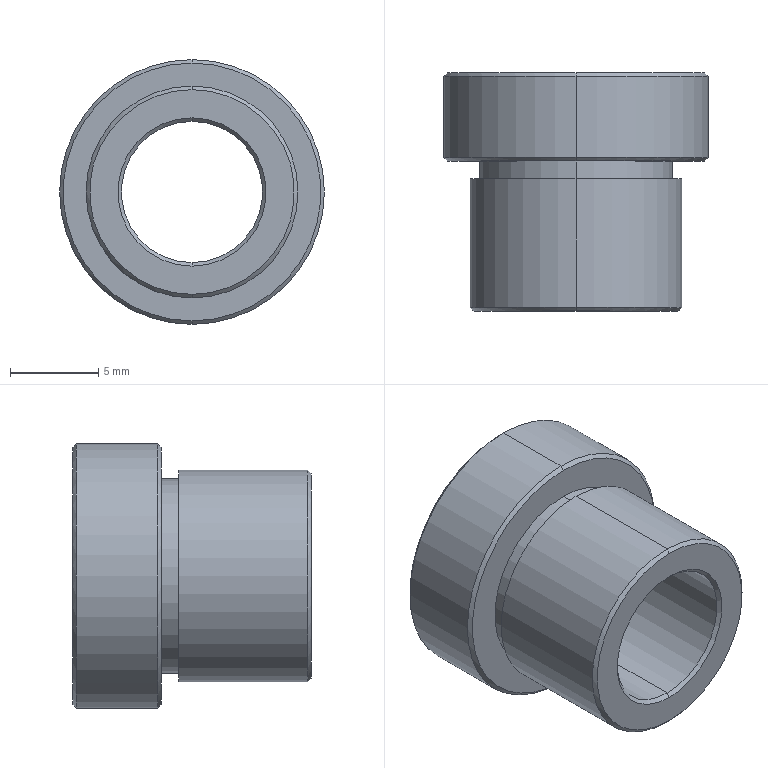Part | STEP file | PN_0020 side positioning guide sleeve_Default | 1 solid | 22 faces | box 15 x 13.5 x 15 mm | volume 1145 mm3 | cone 10 | cylinder 8 | plane 4 | commonest cylinder face diameters 8 x2 11 x2 12 x2 15 x2
STEP:
#1=CARTESIAN_POINT('',(0.,0.,0.));
#2=DIRECTION('',(0.,0.,1.));
#3=DIRECTION('',(1.,0.,0.));
#4=AXIS2_PLACEMENT_3D('',#1,#2,#3);
#5=CARTESIAN_POINT('',(0.,7.5,-5.5));
#6=VERTEX_POINT('',#5);
#7=CARTESIAN_POINT('',(0.,7.5,5.5));
#8=VERTEX_POINT('',#7);
#9=CARTESIAN_POINT('',(0.,7.5,0.));
#10=DIRECTION('',(0.,-1.,0.));
#11=DIRECTION('',(0.,0.,-1.));
#12=AXIS2_PLACEMENT_3D('',#9,#10,#11);
#13=CIRCLE('',#12,5.5);
#14=CARTESIAN_POINT('',(0.,7.5,0.));
#15=DIRECTION('',(0.,1.,0.));
#16=DIRECTION('',(0.,0.,1.));
#17=AXIS2_PLACEMENT_3D('',#14,#15,#16);
#18=CYLINDRICAL_SURFACE('',#17,5.5);
#19=CARTESIAN_POINT('',(3.142,0.));
#20=DIRECTION('',(-1.,0.));
#21=VECTOR('',#20,1.);
#22=LINE('',#19,#21);
#23=(GEOMETRIC_REPRESENTATION_CONTEXT(2)PARAMETRIC_REPRESENTATION_CONTEXT()REPRESENTATION_CONTEXT('',''));
#24=DEFINITIONAL_REPRESENTATION('',(#22),#23);
#25=PCURVE('',#18,#24);
#26=CARTESIAN_POINT('',(0.,7.5,0.));
#27=DIRECTION('',(0.,-1.,0.));
#28=DIRECTION('',(0.,0.,-1.));
#29=AXIS2_PLACEMENT_3D('',#26,#27,#28);
#30=PLANE('',#29);
#31=CARTESIAN_POINT('',(0.,0.));
#32=DIRECTION('',(1.,0.));
#33=AXIS2_PLACEMENT_2D('',#31,#32);
#34=CIRCLE('',#33,5.5);
#35=(GEOMETRIC_REPRESENTATION_CONTEXT(2)PARAMETRIC_REPRESENTATION_CONTEXT()REPRESENTATION_CONTEXT('',''));
#36=DEFINITIONAL_REPRESENTATION('',(#34),#35);
#37=PCURVE('',#30,#36);
#38=SURFACE_CURVE('',#13,(#25,#37),.PCURVE_S1.);
#39=EDGE_CURVE('',#6,#8,#38,.T.);
#40=ORIENTED_EDGE('',*,*,#39,.F.);
#41=CARTESIAN_POINT('',(0.,8.5,-5.5));
#42=VERTEX_POINT('',#41);
#43=CARTESIAN_POINT('',(0.,7.5,-5.5));
#44=DIRECTION('',(0.,1.,0.));
#45=VECTOR('',#44,1.);
#46=LINE('',#43,#45);
#47=CARTESIAN_POINT('',(3.142,0.));
#48=DIRECTION('',(0.,1.));
#49=VECTOR('',#48,1.);
#50=LINE('',#47,#49);
#51=(GEOMETRIC_REPRESENTATION_CONTEXT(2)PARAMETRIC_REPRESENTATION_CONTEXT()REPRESENTATION_CONTEXT('',''));
#52=DEFINITIONAL_REPRESENTATION('',(#50),#51);
#53=PCURVE('',#18,#52);
#54=CARTESIAN_POINT('',(0.,7.5,0.));
#55=DIRECTION('',(0.,1.,0.));
#56=DIRECTION('',(0.,0.,1.));
#57=AXIS2_PLACEMENT_3D('',#54,#55,#56);
#58=CYLINDRICAL_SURFACE('',#57,5.5);
#59=CARTESIAN_POINT('',(3.142,0.));
#60=DIRECTION('',(0.,1.));
#61=VECTOR('',#60,1.);
#62=LINE('',#59,#61);
#63=(GEOMETRIC_REPRESENTATION_CONTEXT(2)PARAMETRIC_REPRESENTATION_CONTEXT()REPRESENTATION_CONTEXT('',''));
#64=DEFINITIONAL_REPRESENTATION('',(#62),#63);
#65=PCURVE('',#58,#64);
#66=SURFACE_CURVE('',#46,(#53,#65),.PCURVE_S1.);
#67=EDGE_CURVE('',#6,#42,#66,.T.);
#68=ORIENTED_EDGE('',*,*,#67,.T.);
#69=CARTESIAN_POINT('',(0.,8.5,5.5));
#70=VERTEX_POINT('',#69);
#71=CARTESIAN_POINT('',(0.,8.5,0.));
#72=DIRECTION('',(0.,-1.,0.));
#73=DIRECTION('',(0.,0.,-1.));
#74=AXIS2_PLACEMENT_3D('',#71,#72,#73);
#75=CIRCLE('',#74,5.5);
#76=CARTESIAN_POINT('',(3.142,1.));
#77=DIRECTION('',(-1.,0.));
#78=VECTOR('',#77,1.);
#79=LINE('',#76,#78);
#80=(GEOMETRIC_REPRESENTATION_CONTEXT(2)PARAMETRIC_REPRESENTATION_CONTEXT()REPRESENTATION_CONTEXT('',''));
#81=DEFINITIONAL_REPRESENTATION('',(#79),#80);
#82=PCURVE('',#18,#81);
#83=CARTESIAN_POINT('',(0.,8.5,0.));
#84=DIRECTION('',(0.,1.,0.));
#85=DIRECTION('',(0.,0.,1.));
#86=AXIS2_PLACEMENT_3D('',#83,#84,#85);
#87=PLANE('',#86);
#88=CARTESIAN_POINT('',(-5.5,0.));
#89=CARTESIAN_POINT('',(-5.5,9.526));
#90=CARTESIAN_POINT('',(2.75,4.763));
#91=CARTESIAN_POINT('',(11.,0.));
#92=CARTESIAN_POINT('',(2.75,-4.763));
#93=CARTESIAN_POINT('',(-5.5,-9.526));
#94=CARTESIAN_POINT('',(-5.5,0.));
#95=(BOUNDED_CURVE()B_SPLINE_CURVE(2,(#88,#89,#90,#91,#92,#93,#94),.UNSPECIFIED.,.T.,.F.)B_SPLINE_CURVE_WITH_KNOTS((1,2,2,2,2,1),(-2.094,0.,2.094,4.189,6.283,8.378),.UNSPECIFIED.)CURVE()GEOMETRIC_REPRESENTATION_ITEM()RATIONAL_B_SPLINE_CURVE((1.,0.5,1.,0.5,1.,0.5,1.))REPRESENTATION_ITEM(''));
#96=(GEOMETRIC_REPRESENTATION_CONTEXT(2)PARAMETRIC_REPRESENTATION_CONTEXT()REPRESENTATION_CONTEXT('',''));
#97=DEFINITIONAL_REPRESENTATION('',(#95),#96);
#98=PCURVE('',#87,#97);
#99=SURFACE_CURVE('',#75,(#82,#98),.PCURVE_S1.);
#100=EDGE_CURVE('',#42,#70,#99,.T.);
#101=ORIENTED_EDGE('',*,*,#100,.T.);
#102=CARTESIAN_POINT('',(0.,7.5,5.5));
#103=DIRECTION('',(0.,1.,0.));
#104=VECTOR('',#103,1.);
#105=LINE('',#102,#104);
#106=CARTESIAN_POINT('',(0.,0.));
#107=DIRECTION('',(0.,1.));
#108=VECTOR('',#107,1.);
#109=LINE('',#106,#108);
#110=(GEOMETRIC_REPRESENTATION_CONTEXT(2)PARAMETRIC_REPRESENTATION_CONTEXT()REPRESENTATION_CONTEXT('',''));
#111=DEFINITIONAL_REPRESENTATION('',(#109),#110);
#112=PCURVE('',#18,#111);
#113=CARTESIAN_POINT('',(6.283,0.));
#114=DIRECTION('',(0.,1.));
#115=VECTOR('',#114,1.);
#116=LINE('',#113,#115);
#117=(GEOMETRIC_REPRESENTATION_CONTEXT(2)PARAMETRIC_REPRESENTATION_CONTEXT()REPRESENTATION_CONTEXT('',''));
#118=DEFINITIONAL_REPRESENTATION('',(#116),#117);
#119=PCURVE('',#58,#118);
#120=SURFACE_CURVE('',#105,(#112,#119),.PCURVE_S1.);
#121=EDGE_CURVE('',#8,#70,#120,.T.);
#122=ORIENTED_EDGE('',*,*,#121,.F.);
#123=EDGE_LOOP('',(#40,#68,#101,#122));
#124=FACE_BOUND('',#123,.T.);
#125=ADVANCED_FACE('',(#124),#18,.T.);
#126=CARTESIAN_POINT('',(0.,13.3,4.));
#127=VERTEX_POINT('',#126);
#128=CARTESIAN_POINT('',(0.,13.5,4.2));
#129=VERTEX_POINT('',#128);
#130=CARTESIAN_POINT('',(0.,13.3,4.));
#131=DIRECTION('',(0.,0.7071,0.7071));
#132=VECTOR('',#131,1.);
#133=LINE('',#130,#132);
#134=CARTESIAN_POINT('',(0.,13.3,0.));
#135=DIRECTION('',(0.,1.,0.));
#136=DIRECTION('',(0.,0.,1.));
#137=AXIS2_PLACEMENT_3D('',#134,#135,#136);
#138=CONICAL_SURFACE('',#137,4.,0.7854);
#139=CARTESIAN_POINT('',(6.283,0.));
#140=DIRECTION('',(0.,1.));
#141=VECTOR('',#140,1.);
#142=LINE('',#139,#141);
#143=(GEOMETRIC_REPRESENTATION_CONTEXT(2)PARAMETRIC_REPRESENTATION_CONTEXT()REPRESENTATION_CONTEXT('',''));
#144=DEFINITIONAL_REPRESENTATION('',(#142),#143);
#145=PCURVE('',#138,#144);
#146=CARTESIAN_POINT('',(0.,13.3,0.));
#147=DIRECTION('',(0.,1.,0.));
#148=DIRECTION('',(0.,0.,1.));
#149=AXIS2_PLACEMENT_3D('',#146,#147,#148);
#150=CONICAL_SURFACE('',#149,4.,0.7854);
#151=CARTESIAN_POINT('',(0.,0.));
#152=DIRECTION('',(0.,1.));
#153=VECTOR('',#152,1.);
#154=LINE('',#151,#153);
#155=(GEOMETRIC_REPRESENTATION_CONTEXT(2)PARAMETRIC_REPRESENTATION_CONTEXT()REPRESENTATION_CONTEXT('',''));
#156=DEFINITIONAL_REPRESENTATION('',(#154),#155);
#157=PCURVE('',#150,#156);
#158=SURFACE_CURVE('',#133,(#145,#157),.PCURVE_S1.);
#159=EDGE_CURVE('',#127,#129,#158,.T.);
#160=ORIENTED_EDGE('',*,*,#159,.T.);
#161=CARTESIAN_POINT('',(0.,13.5,-4.2));
#162=VERTEX_POINT('',#161);
#163=CARTESIAN_POINT('',(0.,13.5,0.));
#164=DIRECTION('',(0.,-1.,0.));
#165=DIRECTION('',(0.,0.,1.));
#166=AXIS2_PLACEMENT_3D('',#163,#164,#165);
#167=CIRCLE('',#166,4.2);
#168=CARTESIAN_POINT('',(6.283,0.2));
#169=DIRECTION('',(-1.,0.));
#170=VECTOR('',#169,1.);
#171=LINE('',#168,#170);
#172=(GEOMETRIC_REPRESENTATION_CONTEXT(2)PARAMETRIC_REPRESENTATION_CONTEXT()REPRESENTATION_CONTEXT('',''));
#173=DEFINITIONAL_REPRESENTATION('',(#171),#172);
#174=PCURVE('',#138,#173);
#175=CARTESIAN_POINT('',(0.,13.5,0.));
#176=DIRECTION('',(0.,1.,0.));
#177=DIRECTION('',(0.,0.,1.));
#178=AXIS2_PLACEMENT_3D('',#175,#176,#177);
#179=PLANE('',#178);
#180=CARTESIAN_POINT('',(4.2,0.));
#181=CARTESIAN_POINT('',(4.2,-7.275));
#182=CARTESIAN_POINT('',(-2.1,-3.637));
#183=CARTESIAN_POINT('',(-8.4,0.));
#184=CARTESIAN_POINT('',(-2.1,3.637));
#185=CARTESIAN_POINT('',(4.2,7.275));
#186=CARTESIAN_POINT('',(4.2,0.));
#187=(BOUNDED_CURVE()B_SPLINE_CURVE(2,(#180,#181,#182,#183,#184,#185,#186),.UNSPECIFIED.,.T.,.F.)B_SPLINE_CURVE_WITH_KNOTS((1,2,2,2,2,1),(-2.094,0.,2.094,4.189,6.283,8.378),.UNSPECIFIED.)CURVE()GEOMETRIC_REPRESENTATION_ITEM()RATIONAL_B_SPLINE_CURVE((1.,0.5,1.,0.5,1.,0.5,1.))REPRESENTATION_ITEM(''));
#188=(GEOMETRIC_REPRESENTATION_CONTEXT(2)PARAMETRIC_REPRESENTATION_CONTEXT()REPRESENTATION_CONTEXT('',''));
#189=DEFINITIONAL_REPRESENTATION('',(#187),#188);
#190=PCURVE('',#179,#189);
#191=SURFACE_CURVE('',#167,(#174,#190),.PCURVE_S1.);
#192=EDGE_CURVE('',#129,#162,#191,.T.);
#193=ORIENTED_EDGE('',*,*,#192,.T.);
#194=CARTESIAN_POINT('',(0.,13.3,-4.));
#195=VERTEX_POINT('',#194);
#196=CARTESIAN_POINT('',(0.,13.3,-4.));
#197=DIRECTION('',(0.,0.7071,-0.7071));
#198=VECTOR('',#197,1.);
#199=LINE('',#196,#198);
#200=CARTESIAN_POINT('',(3.142,0.));
#201=DIRECTION('',(0.,1.));
#202=VECTOR('',#201,1.);
#203=LINE('',#200,#202);
#204=(GEOMETRIC_REPRESENTATION_CONTEXT(2)PARAMETRIC_REPRESENTATION_CONTEXT()REPRESENTATION_CONTEXT('',''));
#205=DEFINITIONAL_REPRESENTATION('',(#203),#204);
#206=PCURVE('',#138,#205);
#207=CARTESIAN_POINT('',(3.142,0.));
#208=DIRECTION('',(0.,1.));
#209=VECTOR('',#208,1.);
#210=LINE('',#207,#209);
#211=(GEOMETRIC_REPRESENTATION_CONTEXT(2)PARAMETRIC_REPRESENTATION_CONTEXT()REPRESENTATION_CONTEXT('',''));
#212=DEFINITIONAL_REPRESENTATION('',(#210),#211);
#213=PCURVE('',#150,#212);
#214=SURFACE_CURVE('',#199,(#206,#213),.PCURVE_S1.);
#215=EDGE_CURVE('',#195,#162,#214,.T.);
#216=ORIENTED_EDGE('',*,*,#215,.F.);
#217=CARTESIAN_POINT('',(0.,13.3,0.));
#218=DIRECTION('',(0.,1.,0.));
#219=DIRECTION('',(0.,0.,1.));
#220=AXIS2_PLACEMENT_3D('',#217,#218,#219);
#221=CIRCLE('',#220,4.);
#222=CARTESIAN_POINT('',(0.,0.));
#223=DIRECTION('',(1.,0.));
#224=VECTOR('',#223,1.);
#225=LINE('',#222,#224);
#226=(GEOMETRIC_REPRESENTATION_CONTEXT(2)PARAMETRIC_REPRESENTATION_CONTEXT()REPRESENTATION_CONTEXT('',''));
#227=DEFINITIONAL_REPRESENTATION('',(#225),#226);
#228=PCURVE('',#138,#227);
#229=CARTESIAN_POINT('',(0.,8.5,0.));
#230=DIRECTION('',(0.,-1.,0.));
#231=DIRECTION('',(0.,0.,-1.));
#232=AXIS2_PLACEMENT_3D('',#229,#230,#231);
#233=CYLINDRICAL_SURFACE('',#232,4.);
#234=CARTESIAN_POINT('',(9.425,-4.8));
#235=DIRECTION('',(-1.,0.));
#236=VECTOR('',#235,1.);
#237=LINE('',#234,#236);
#238=(GEOMETRIC_REPRESENTATION_CONTEXT(2)PARAMETRIC_REPRESENTATION_CONTEXT()REPRESENTATION_CONTEXT('',''));
#239=DEFINITIONAL_REPRESENTATION('',(#237),#238);
#240=PCURVE('',#233,#239);
#241=SURFACE_CURVE('',#221,(#228,#240),.PCURVE_S1.);
#242=EDGE_CURVE('',#195,#127,#241,.T.);
#243=ORIENTED_EDGE('',*,*,#242,.T.);
#244=EDGE_LOOP('',(#160,#193,#216,#243));
#245=FACE_BOUND('',#244,.F.);
#246=ADVANCED_FACE('',(#245),#138,.F.);
#247=CARTESIAN_POINT('',(0.,13.5,7.3));
#248=VERTEX_POINT('',#247);
#249=CARTESIAN_POINT('',(0.,13.5,-7.3));
#250=VERTEX_POINT('',#249);
#251=CARTESIAN_POINT('',(0.,13.5,0.));
#252=DIRECTION('',(0.,1.,0.));
#253=DIRECTION('',(0.,0.,1.));
#254=AXIS2_PLACEMENT_3D('',#251,#252,#253);
#255=CIRCLE('',#254,7.3);
#256=CARTESIAN_POINT('',(0.,13.5,0.));
#257=DIRECTION('',(0.,-1.,0.));
#258=DIRECTION('',(0.,0.,-1.));
#259=AXIS2_PLACEMENT_3D('',#256,#257,#258);
#260=CONICAL_SURFACE('',#259,7.3,0.7854);
#261=CARTESIAN_POINT('',(3.142,0.));
#262=DIRECTION('',(-1.,0.));
#263=VECTOR('',#262,1.);
#264=LINE('',#261,#263);
#265=(GEOMETRIC_REPRESENTATION_CONTEXT(2)PARAMETRIC_REPRESENTATION_CONTEXT()REPRESENTATION_CONTEXT('',''));
#266=DEFINITIONAL_REPRESENTATION('',(#264),#265);
#267=PCURVE('',#260,#266);
#268=CARTESIAN_POINT('',(0.,0.));
#269=DIRECTION('',(1.,0.));
#270=AXIS2_PLACEMENT_2D('',#268,#269);
#271=CIRCLE('',#270,7.3);
#272=(GEOMETRIC_REPRESENTATION_CONTEXT(2)PARAMETRIC_REPRESENTATION_CONTEXT()REPRESENTATION_CONTEXT('',''));
#273=DEFINITIONAL_REPRESENTATION('',(#271),#272);
#274=PCURVE('',#179,#273);
#275=SURFACE_CURVE('',#255,(#267,#274),.PCURVE_S1.);
#276=EDGE_CURVE('',#248,#250,#275,.T.);
#277=ORIENTED_EDGE('',*,*,#276,.F.);
#278=CARTESIAN_POINT('',(0.,13.3,7.5));
#279=VERTEX_POINT('',#278);
#280=CARTESIAN_POINT('',(0.,13.5,7.3));
#281=DIRECTION('',(0.,-0.7071,0.7071));
#282=VECTOR('',#281,1.);
#283=LINE('',#280,#282);
#284=CARTESIAN_POINT('',(3.142,0.));
#285=DIRECTION('',(0.,1.));
#286=VECTOR('',#285,1.);
#287=LINE('',#284,#286);
#288=(GEOMETRIC_REPRESENTATION_CONTEXT(2)PARAMETRIC_REPRESENTATION_CONTEXT()REPRESENTATION_CONTEXT('',''));
#289=DEFINITIONAL_REPRESENTATION('',(#287),#288);
#290=PCURVE('',#260,#289);
#291=CARTESIAN_POINT('',(0.,13.5,0.));
#292=DIRECTION('',(0.,-1.,0.));
#293=DIRECTION('',(0.,0.,-1.));
#294=AXIS2_PLACEMENT_3D('',#291,#292,#293);
#295=CONICAL_SURFACE('',#294,7.3,0.7854);
#296=CARTESIAN_POINT('',(3.142,0.));
#297=DIRECTION('',(0.,1.));
#298=VECTOR('',#297,1.);
#299=LINE('',#296,#298);
#300=(GEOMETRIC_REPRESENTATION_CONTEXT(2)PARAMETRIC_REPRESENTATION_CONTEXT()REPRESENTATION_CONTEXT('',''));
#301=DEFINITIONAL_REPRESENTATION('',(#299),#300);
#302=PCURVE('',#295,#301);
#303=SURFACE_CURVE('',#283,(#290,#302),.PCURVE_S1.);
#304=EDGE_CURVE('',#248,#279,#303,.T.);
#305=ORIENTED_EDGE('',*,*,#304,.T.);
#306=CARTESIAN_POINT('',(0.,13.3,-7.5));
#307=VERTEX_POINT('',#306);
#308=CARTESIAN_POINT('',(0.,13.3,0.));
#309=DIRECTION('',(0.,-1.,0.));
#310=DIRECTION('',(0.,0.,1.));
#311=AXIS2_PLACEMENT_3D('',#308,#309,#310);
#312=CIRCLE('',#311,7.5);
#313=CARTESIAN_POINT('',(-3.142,0.2));
#314=DIRECTION('',(1.,0.));
#315=VECTOR('',#314,1.);
#316=LINE('',#313,#315);
#317=(GEOMETRIC_REPRESENTATION_CONTEXT(2)PARAMETRIC_REPRESENTATION_CONTEXT()REPRESENTATION_CONTEXT('',''));
#318=DEFINITIONAL_REPRESENTATION('',(#316),#317);
#319=PCURVE('',#260,#318);
#320=CARTESIAN_POINT('',(0.,13.5,0.));
#321=DIRECTION('',(0.,-1.,0.));
#322=DIRECTION('',(0.,0.,-1.));
#323=AXIS2_PLACEMENT_3D('',#320,#321,#322);
#324=CYLINDRICAL_SURFACE('',#323,7.5);
#325=CARTESIAN_POINT('',(-3.142,0.2));
#326=DIRECTION('',(1.,0.));
#327=VECTOR('',#326,1.);
#328=LINE('',#325,#327);
#329=(GEOMETRIC_REPRESENTATION_CONTEXT(2)PARAMETRIC_REPRESENTATION_CONTEXT()REPRESENTATION_CONTEXT('',''));
#330=DEFINITIONAL_REPRESENTATION('',(#328),#329);
#331=PCURVE('',#324,#330);
#332=SURFACE_CURVE('',#312,(#319,#331),.PCURVE_S1.);
#333=EDGE_CURVE('',#307,#279,#332,.T.);
#334=ORIENTED_EDGE('',*,*,#333,.F.);
#335=CARTESIAN_POINT('',(0.,13.5,-7.3));
#336=DIRECTION('',(0.,-0.7071,-0.7071));
#337=VECTOR('',#336,1.);
#338=LINE('',#335,#337);
#339=CARTESIAN_POINT('',(0.,0.));
#340=DIRECTION('',(0.,1.));
#341=VECTOR('',#340,1.);
#342=LINE('',#339,#341);
#343=(GEOMETRIC_REPRESENTATION_CONTEXT(2)PARAMETRIC_REPRESENTATION_CONTEXT()REPRESENTATION_CONTEXT('',''));
#344=DEFINITIONAL_REPRESENTATION('',(#342),#343);
#345=PCURVE('',#260,#344);
#346=CARTESIAN_POINT('',(6.283,0.));
#347=DIRECTION('',(0.,1.));
#348=VECTOR('',#347,1.);
#349=LINE('',#346,#348);
#350=(GEOMETRIC_REPRESENTATION_CONTEXT(2)PARAMETRIC_REPRESENTATION_CONTEXT()REPRESENTATION_CONTEXT('',''));
#351=DEFINITIONAL_REPRESENTATION('',(#349),#350);
#352=PCURVE('',#295,#351);
#353=SURFACE_CURVE('',#338,(#345,#352),.PCURVE_S1.);
#354=EDGE_CURVE('',#250,#307,#353,.T.);
#355=ORIENTED_EDGE('',*,*,#354,.F.);
#356=EDGE_LOOP('',(#277,#305,#334,#355));
#357=FACE_BOUND('',#356,.T.);
#358=ADVANCED_FACE('',(#357),#260,.T.);
#359=CARTESIAN_POINT('',(0.,8.5,-7.3));
#360=VERTEX_POINT('',#359);
#361=CARTESIAN_POINT('',(0.,8.5,7.3));
#362=VERTEX_POINT('',#361);
#363=CARTESIAN_POINT('',(0.,8.5,0.));
#364=DIRECTION('',(0.,-1.,0.));
#365=DIRECTION('',(0.,0.,1.));
#366=AXIS2_PLACEMENT_3D('',#363,#364,#365);
#367=CIRCLE('',#366,7.3);
#368=CARTESIAN_POINT('',(0.,8.7,0.));
#369=DIRECTION('',(0.,1.,0.));
#370=DIRECTION('',(0.,0.,1.));
#371=AXIS2_PLACEMENT_3D('',#368,#369,#370);
#372=CONICAL_SURFACE('',#371,7.5,0.7854);
#373=CARTESIAN_POINT('',(6.283,-0.2));
#374=DIRECTION('',(-1.,0.));
#375=VECTOR('',#374,1.);
#376=LINE('',#373,#375);
#377=(GEOMETRIC_REPRESENTATION_CONTEXT(2)PARAMETRIC_REPRESENTATION_CONTEXT()REPRESENTATION_CONTEXT('',''));
#378=DEFINITIONAL_REPRESENTATION('',(#376),#377);
#379=PCURVE('',#372,#378);
#380=CARTESIAN_POINT('',(7.3,0.));
#381=CARTESIAN_POINT('',(7.3,-12.644));
#382=CARTESIAN_POINT('',(-3.65,-6.322));
#383=CARTESIAN_POINT('',(-14.6,0.));
#384=CARTESIAN_POINT('',(-3.65,6.322));
#385=CARTESIAN_POINT('',(7.3,12.644));
#386=CARTESIAN_POINT('',(7.3,0.));
#387=(BOUNDED_CURVE()B_SPLINE_CURVE(2,(#380,#381,#382,#383,#384,#385,#386),.UNSPECIFIED.,.T.,.F.)B_SPLINE_CURVE_WITH_KNOTS((1,2,2,2,2,1),(-2.094,0.,2.094,4.189,6.283,8.378),.UNSPECIFIED.)CURVE()GEOMETRIC_REPRESENTATION_ITEM()RATIONAL_B_SPLINE_CURVE((1.,0.5,1.,0.5,1.,0.5,1.))REPRESENTATION_ITEM(''));
#388=(GEOMETRIC_REPRESENTATION_CONTEXT(2)PARAMETRIC_REPRESENTATION_CONTEXT()REPRESENTATION_CONTEXT('',''));
#389=DEFINITIONAL_REPRESENTATION('',(#387),#388);
#390=PCURVE('',#87,#389);
#391=SURFACE_CURVE('',#367,(#379,#390),.PCURVE_S1.);
#392=EDGE_CURVE('',#360,#362,#391,.T.);
#393=ORIENTED_EDGE('',*,*,#392,.F.);
#394=CARTESIAN_POINT('',(0.,8.7,-7.5));
#395=VERTEX_POINT('',#394);
#396=CARTESIAN_POINT('',(0.,8.7,-7.5));
#397=DIRECTION('',(0.,0.7071,-0.7071));
#398=VECTOR('',#397,1.);
#399=LINE('',#396,#398);
#400=CARTESIAN_POINT('',(3.142,0.));
#401=DIRECTION('',(0.,1.));
#402=VECTOR('',#401,1.);
#403=LINE('',#400,#402);
#404=(GEOMETRIC_REPRESENTATION_CONTEXT(2)PARAMETRIC_REPRESENTATION_CONTEXT()REPRESENTATION_CONTEXT('',''));
#405=DEFINITIONAL_REPRESENTATION('',(#403),#404);
#406=PCURVE('',#372,#405);
#407=CARTESIAN_POINT('',(0.,8.7,0.));
#408=DIRECTION('',(0.,1.,0.));
#409=DIRECTION('',(0.,0.,1.));
#410=AXIS2_PLACEMENT_3D('',#407,#408,#409);
#411=CONICAL_SURFACE('',#410,7.5,0.7854);
#412=CARTESIAN_POINT('',(3.142,0.));
#413=DIRECTION('',(0.,1.));
#414=VECTOR('',#413,1.);
#415=LINE('',#412,#414);
#416=(GEOMETRIC_REPRESENTATION_CONTEXT(2)PARAMETRIC_REPRESENTATION_CONTEXT()REPRESENTATION_CONTEXT('',''));
#417=DEFINITIONAL_REPRESENTATION('',(#415),#416);
#418=PCURVE('',#411,#417);
#419=SURFACE_CURVE('',#399,(#406,#418),.PCURVE_S1.);
#420=EDGE_CURVE('',#360,#395,#419,.T.);
#421=ORIENTED_EDGE('',*,*,#420,.T.);
#422=CARTESIAN_POINT('',(0.,8.7,7.5));
#423=VERTEX_POINT('',#422);
#424=CARTESIAN_POINT('',(0.,8.7,0.));
#425=DIRECTION('',(0.,1.,0.));
#426=DIRECTION('',(0.,0.,1.));
#427=AXIS2_PLACEMENT_3D('',#424,#425,#426);
#428=CIRCLE('',#427,7.5);
#429=CARTESIAN_POINT('',(0.,0.));
#430=DIRECTION('',(1.,0.));
#431=VECTOR('',#430,1.);
#432=LINE('',#429,#431);
#433=(GEOMETRIC_REPRESENTATION_CONTEXT(2)PARAMETRIC_REPRESENTATION_CONTEXT()REPRESENTATION_CONTEXT('',''));
#434=DEFINITIONAL_REPRESENTATION('',(#432),#433);
#435=PCURVE('',#372,#434);
#436=CARTESIAN_POINT('',(3.142,4.8));
#437=DIRECTION('',(-1.,0.));
#438=VECTOR('',#437,1.);
#439=LINE('',#436,#438);
#440=(GEOMETRIC_REPRESENTATION_CONTEXT(2)PARAMETRIC_REPRESENTATION_CONTEXT()REPRESENTATION_CONTEXT('',''));
#441=DEFINITIONAL_REPRESENTATION('',(#439),#440);
#442=PCURVE('',#324,#441);
#443=SURFACE_CURVE('',#428,(#435,#442),.PCURVE_S1.);
#444=EDGE_CURVE('',#423,#395,#443,.T.);
#445=ORIENTED_EDGE('',*,*,#444,.F.);
#446=CARTESIAN_POINT('',(0.,8.7,7.5));
#447=DIRECTION('',(0.,0.7071,0.7071));
#448=VECTOR('',#447,1.);
#449=LINE('',#446,#448);
#450=CARTESIAN_POINT('',(0.,0.));
#451=DIRECTION('',(0.,1.));
#452=VECTOR('',#451,1.);
#453=LINE('',#450,#452);
#454=(GEOMETRIC_REPRESENTATION_CONTEXT(2)PARAMETRIC_REPRESENTATION_CONTEXT()REPRESENTATION_CONTEXT('',''));
#455=DEFINITIONAL_REPRESENTATION('',(#453),#454);
#456=PCURVE('',#372,#455);
#457=CARTESIAN_POINT('',(6.283,0.));
#458=DIRECTION('',(0.,1.));
#459=VECTOR('',#458,1.);
#460=LINE('',#457,#459);
#461=(GEOMETRIC_REPRESENTATION_CONTEXT(2)PARAMETRIC_REPRESENTATION_CONTEXT()REPRESENTATION_CONTEXT('',''));
#462=DEFINITIONAL_REPRESENTATION('',(#460),#461);
#463=PCURVE('',#411,#462);
#464=SURFACE_CURVE('',#449,(#456,#463),.PCURVE_S1.);
#465=EDGE_CURVE('',#362,#423,#464,.T.);
#466=ORIENTED_EDGE('',*,*,#465,.F.);
#467=EDGE_LOOP('',(#393,#421,#445,#466));
#468=FACE_BOUND('',#467,.T.);
#469=ADVANCED_FACE('',(#468),#372,.T.);
#470=CARTESIAN_POINT('',(0.,0.,-5.8));
#471=VERTEX_POINT('',#470);
#472=CARTESIAN_POINT('',(0.,0.,5.8));
#473=VERTEX_POINT('',#472);
#474=CARTESIAN_POINT('',(0.,0.,0.));
#475=DIRECTION('',(0.,-1.,0.));
#476=DIRECTION('',(0.,0.,1.));
#477=AXIS2_PLACEMENT_3D('',#474,#475,#476);
#478=CIRCLE('',#477,5.8);
#479=CARTESIAN_POINT('',(0.,0.2,0.));
#480=DIRECTION('',(0.,1.,0.));
#481=DIRECTION('',(0.,0.,1.));
#482=AXIS2_PLACEMENT_3D('',#479,#480,#481);
#483=CONICAL_SURFACE('',#482,6.,0.7854);
#484=CARTESIAN_POINT('',(6.283,-0.2));
#485=DIRECTION('',(-1.,0.));
#486=VECTOR('',#485,1.);
#487=LINE('',#484,#486);
#488=(GEOMETRIC_REPRESENTATION_CONTEXT(2)PARAMETRIC_REPRESENTATION_CONTEXT()REPRESENTATION_CONTEXT('',''));
#489=DEFINITIONAL_REPRESENTATION('',(#487),#488);
#490=PCURVE('',#483,#489);
#491=CARTESIAN_POINT('',(0.,0.,0.));
#492=DIRECTION('',(0.,1.,0.));
#493=DIRECTION('',(0.,0.,1.));
#494=AXIS2_PLACEMENT_3D('',#491,#492,#493);
#495=PLANE('',#494);
#496=CARTESIAN_POINT('',(5.8,0.));
#497=CARTESIAN_POINT('',(5.8,-10.046));
#498=CARTESIAN_POINT('',(-2.9,-5.023));
#499=CARTESIAN_POINT('',(-11.6,0.));
#500=CARTESIAN_POINT('',(-2.9,5.023));
#501=CARTESIAN_POINT('',(5.8,10.046));
#502=CARTESIAN_POINT('',(5.8,0.));
#503=(BOUNDED_CURVE()B_SPLINE_CURVE(2,(#496,#497,#498,#499,#500,#501,#502),.UNSPECIFIED.,.T.,.F.)B_SPLINE_CURVE_WITH_KNOTS((1,2,2,2,2,1),(-2.094,0.,2.094,4.189,6.283,8.378),.UNSPECIFIED.)CURVE()GEOMETRIC_REPRESENTATION_ITEM()RATIONAL_B_SPLINE_CURVE((1.,0.5,1.,0.5,1.,0.5,1.))REPRESENTATION_ITEM(''));
#504=(GEOMETRIC_REPRESENTATION_CONTEXT(2)PARAMETRIC_REPRESENTATION_CONTEXT()REPRESENTATION_CONTEXT('',''));
#505=DEFINITIONAL_REPRESENTATION('',(#503),#504);
#506=PCURVE('',#495,#505);
#507=SURFACE_CURVE('',#478,(#490,#506),.PCURVE_S1.);
#508=EDGE_CURVE('',#471,#473,#507,.T.);
#509=ORIENTED_EDGE('',*,*,#508,.F.);
#510=CARTESIAN_POINT('',(0.,0.2,-6.));
#511=VERTEX_POINT('',#510);
#512=CARTESIAN_POINT('',(0.,0.2,-6.));
#513=DIRECTION('',(0.,0.7071,-0.7071));
#514=VECTOR('',#513,1.);
#515=LINE('',#512,#514);
#516=CARTESIAN_POINT('',(3.142,0.));
#517=DIRECTION('',(0.,1.));
#518=VECTOR('',#517,1.);
#519=LINE('',#516,#518);
#520=(GEOMETRIC_REPRESENTATION_CONTEXT(2)PARAMETRIC_REPRESENTATION_CONTEXT()REPRESENTATION_CONTEXT('',''));
#521=DEFINITIONAL_REPRESENTATION('',(#519),#520);
#522=PCURVE('',#483,#521);
#523=CARTESIAN_POINT('',(0.,0.2,0.));
#524=DIRECTION('',(0.,1.,0.));
#525=DIRECTION('',(0.,0.,1.));
#526=AXIS2_PLACEMENT_3D('',#523,#524,#525);
#527=CONICAL_SURFACE('',#526,6.,0.7854);
#528=CARTESIAN_POINT('',(3.142,0.));
#529=DIRECTION('',(0.,1.));
#530=VECTOR('',#529,1.);
#531=LINE('',#528,#530);
#532=(GEOMETRIC_REPRESENTATION_CONTEXT(2)PARAMETRIC_REPRESENTATION_CONTEXT()REPRESENTATION_CONTEXT('',''));
#533=DEFINITIONAL_REPRESENTATION('',(#531),#532);
#534=PCURVE('',#527,#533);
#535=SURFACE_CURVE('',#515,(#522,#534),.PCURVE_S1.);
#536=EDGE_CURVE('',#471,#511,#535,.T.);
#537=ORIENTED_EDGE('',*,*,#536,.T.);
#538=CARTESIAN_POINT('',(0.,0.2,6.));
#539=VERTEX_POINT('',#538);
#540=CARTESIAN_POINT('',(0.,0.2,0.));
#541=DIRECTION('',(0.,1.,0.));
#542=DIRECTION('',(0.,0.,1.));
#543=AXIS2_PLACEMENT_3D('',#540,#541,#542);
#544=CIRCLE('',#543,6.);
#545=CARTESIAN_POINT('',(0.,0.));
#546=DIRECTION('',(1.,0.));
#547=VECTOR('',#546,1.);
#548=LINE('',#545,#547);
#549=(GEOMETRIC_REPRESENTATION_CONTEXT(2)PARAMETRIC_REPRESENTATION_CONTEXT()REPRESENTATION_CONTEXT('',''));
#550=DEFINITIONAL_REPRESENTATION('',(#548),#549);
#551=PCURVE('',#483,#550);
#552=CARTESIAN_POINT('',(0.,8.5,0.));
#553=DIRECTION('',(0.,-1.,0.));
#554=DIRECTION('',(0.,0.,-1.));
#555=AXIS2_PLACEMENT_3D('',#552,#553,#554);
#556=CYLINDRICAL_SURFACE('',#555,6.);
#557=CARTESIAN_POINT('',(3.142,8.3));
#558=DIRECTION('',(-1.,0.));
#559=VECTOR('',#558,1.);
#560=LINE('',#557,#559);
#561=(GEOMETRIC_REPRESENTATION_CONTEXT(2)PARAMETRIC_REPRESENTATION_CONTEXT()REPRESENTATION_CONTEXT('',''));
#562=DEFINITIONAL_REPRESENTATION('',(#560),#561);
#563=PCURVE('',#556,#562);
#564=SURFACE_CURVE('',#544,(#551,#563),.PCURVE_S1.);
#565=EDGE_CURVE('',#539,#511,#564,.T.);
#566=ORIENTED_EDGE('',*,*,#565,.F.);
#567=CARTESIAN_POINT('',(0.,0.2,6.));
#568=DIRECTION('',(0.,0.7071,0.7071));
#569=VECTOR('',#568,1.);
#570=LINE('',#567,#569);
#571=CARTESIAN_POINT('',(0.,0.));
#572=DIRECTION('',(0.,1.));
#573=VECTOR('',#572,1.);
#574=LINE('',#571,#573);
#575=(GEOMETRIC_REPRESENTATION_CONTEXT(2)PARAMETRIC_REPRESENTATION_CONTEXT()REPRESENTATION_CONTEXT('',''));
#576=DEFINITIONAL_REPRESENTATION('',(#574),#575);
#577=PCURVE('',#483,#576);
#578=CARTESIAN_POINT('',(6.283,0.));
#579=DIRECTION('',(0.,1.));
#580=VECTOR('',#579,1.);
#581=LINE('',#578,#580);
#582=(GEOMETRIC_REPRESENTATION_CONTEXT(2)PARAMETRIC_REPRESENTATION_CONTEXT()REPRESENTATION_CONTEXT('',''));
#583=DEFINITIONAL_REPRESENTATION('',(#581),#582);
#584=PCURVE('',#527,#583);
#585=SURFACE_CURVE('',#570,(#577,#584),.PCURVE_S1.);
#586=EDGE_CURVE('',#473,#539,#585,.T.);
#587=ORIENTED_EDGE('',*,*,#586,.F.);
#588=EDGE_LOOP('',(#509,#537,#566,#587));
#589=FACE_BOUND('',#588,.T.);
#590=ADVANCED_FACE('',(#589),#483,.T.);
#591=CARTESIAN_POINT('',(0.,0.2,-4.));
#592=VERTEX_POINT('',#591);
#593=CARTESIAN_POINT('',(0.,0.,-4.2));
#594=VERTEX_POINT('',#593);
#595=CARTESIAN_POINT('',(0.,0.,-4.2));
#596=DIRECTION('',(0.,-0.7071,-0.7071));
#597=VECTOR('',#596,1.);
#598=LINE('',#595,#597);
#599=CARTESIAN_POINT('',(0.,0.,0.));
#600=DIRECTION('',(0.,-1.,0.));
#601=DIRECTION('',(0.,0.,-1.));
#602=AXIS2_PLACEMENT_3D('',#599,#600,#601);
#603=CONICAL_SURFACE('',#602,4.2,0.7854);
#604=CARTESIAN_POINT('',(6.283,0.));
#605=DIRECTION('',(0.,1.));
#606=VECTOR('',#605,1.);
#607=LINE('',#604,#606);
#608=(GEOMETRIC_REPRESENTATION_CONTEXT(2)PARAMETRIC_REPRESENTATION_CONTEXT()REPRESENTATION_CONTEXT('',''));
#609=DEFINITIONAL_REPRESENTATION('',(#607),#608);
#610=PCURVE('',#603,#609);
#611=CARTESIAN_POINT('',(0.,0.,0.));
#612=DIRECTION('',(0.,-1.,0.));
#613=DIRECTION('',(0.,0.,-1.));
#614=AXIS2_PLACEMENT_3D('',#611,#612,#613);
#615=CONICAL_SURFACE('',#614,4.2,0.7854);
#616=CARTESIAN_POINT('',(0.,0.));
#617=DIRECTION('',(0.,1.));
#618=VECTOR('',#617,1.);
#619=LINE('',#616,#618);
#620=(GEOMETRIC_REPRESENTATION_CONTEXT(2)PARAMETRIC_REPRESENTATION_CONTEXT()REPRESENTATION_CONTEXT('',''));
#621=DEFINITIONAL_REPRESENTATION('',(#619),#620);
#622=PCURVE('',#615,#621);
#623=SURFACE_CURVE('',#598,(#610,#622),.PCURVE_S1.);
#624=EDGE_CURVE('',#592,#594,#623,.T.);
#625=ORIENTED_EDGE('',*,*,#624,.T.);
#626=CARTESIAN_POINT('',(0.,0.,4.2));
#627=VERTEX_POINT('',#626);
#628=CARTESIAN_POINT('',(0.,0.,0.));
#629=DIRECTION('',(0.,1.,0.));
#630=DIRECTION('',(0.,0.,1.));
#631=AXIS2_PLACEMENT_3D('',#628,#629,#630);
#632=CIRCLE('',#631,4.2);
#633=CARTESIAN_POINT('',(9.425,0.));
#634=DIRECTION('',(-1.,0.));
#635=VECTOR('',#634,1.);
#636=LINE('',#633,#635);
#637=(GEOMETRIC_REPRESENTATION_CONTEXT(2)PARAMETRIC_REPRESENTATION_CONTEXT()REPRESENTATION_CONTEXT('',''));
#638=DEFINITIONAL_REPRESENTATION('',(#636),#637);
#639=PCURVE('',#603,#638);
#640=CARTESIAN_POINT('',(0.,0.));
#641=DIRECTION('',(1.,0.));
#642=AXIS2_PLACEMENT_2D('',#640,#641);
#643=CIRCLE('',#642,4.2);
#644=(GEOMETRIC_REPRESENTATION_CONTEXT(2)PARAMETRIC_REPRESENTATION_CONTEXT()REPRESENTATION_CONTEXT('',''));
#645=DEFINITIONAL_REPRESENTATION('',(#643),#644);
#646=PCURVE('',#495,#645);
#647=SURFACE_CURVE('',#632,(#639,#646),.PCURVE_S1.);
#648=EDGE_CURVE('',#594,#627,#647,.T.);
#649=ORIENTED_EDGE('',*,*,#648,.T.);
#650=CARTESIAN_POINT('',(0.,0.2,4.));
#651=VERTEX_POINT('',#650);
#652=CARTESIAN_POINT('',(0.,0.,4.2));
#653=DIRECTION('',(0.,-0.7071,0.7071));
#654=VECTOR('',#653,1.);
#655=LINE('',#652,#654);
#656=CARTESIAN_POINT('',(3.142,0.));
#657=DIRECTION('',(0.,1.));
#658=VECTOR('',#657,1.);
#659=LINE('',#656,#658);
#660=(GEOMETRIC_REPRESENTATION_CONTEXT(2)PARAMETRIC_REPRESENTATION_CONTEXT()REPRESENTATION_CONTEXT('',''));
#661=DEFINITIONAL_REPRESENTATION('',(#659),#660);
#662=PCURVE('',#603,#661);
#663=CARTESIAN_POINT('',(3.142,0.));
#664=DIRECTION('',(0.,1.));
#665=VECTOR('',#664,1.);
#666=LINE('',#663,#665);
#667=(GEOMETRIC_REPRESENTATION_CONTEXT(2)PARAMETRIC_REPRESENTATION_CONTEXT()REPRESENTATION_CONTEXT('',''));
#668=DEFINITIONAL_REPRESENTATION('',(#666),#667);
#669=PCURVE('',#615,#668);
#670=SURFACE_CURVE('',#655,(#662,#669),.PCURVE_S1.);
#671=EDGE_CURVE('',#651,#627,#670,.T.);
#672=ORIENTED_EDGE('',*,*,#671,.F.);
#673=CARTESIAN_POINT('',(0.,0.2,0.));
#674=DIRECTION('',(0.,-1.,0.));
#675=DIRECTION('',(0.,0.,1.));
#676=AXIS2_PLACEMENT_3D('',#673,#674,#675);
#677=CIRCLE('',#676,4.);
#678=CARTESIAN_POINT('',(3.142,-0.2));
#679=DIRECTION('',(1.,0.));
#680=VECTOR('',#679,1.);
#681=LINE('',#678,#680);
#682=(GEOMETRIC_REPRESENTATION_CONTEXT(2)PARAMETRIC_REPRESENTATION_CONTEXT()REPRESENTATION_CONTEXT('',''));
#683=DEFINITIONAL_REPRESENTATION('',(#681),#682);
#684=PCURVE('',#603,#683);
#685=CARTESIAN_POINT('',(3.142,8.3));
#686=DIRECTION('',(1.,0.));
#687=VECTOR('',#686,1.);
#688=LINE('',#685,#687);
#689=(GEOMETRIC_REPRESENTATION_CONTEXT(2)PARAMETRIC_REPRESENTATION_CONTEXT()REPRESENTATION_CONTEXT('',''));
#690=DEFINITIONAL_REPRESENTATION('',(#688),#689);
#691=PCURVE('',#233,#690);
#692=SURFACE_CURVE('',#677,(#684,#691),.PCURVE_S1.);
#693=EDGE_CURVE('',#651,#592,#692,.T.);
#694=ORIENTED_EDGE('',*,*,#693,.T.);
#695=EDGE_LOOP('',(#625,#649,#672,#694));
#696=FACE_BOUND('',#695,.F.);
#697=ADVANCED_FACE('',(#696),#603,.F.);
#698=ORIENTED_EDGE('',*,*,#333,.T.);
#699=CARTESIAN_POINT('',(0.,13.5,7.5));
#700=DIRECTION('',(0.,-1.,0.));
#701=VECTOR('',#700,1.);
#702=LINE('',#699,#701);
#703=CARTESIAN_POINT('',(3.142,0.));
#704=DIRECTION('',(0.,1.));
#705=VECTOR('',#704,1.);
#706=LINE('',#703,#705);
#707=(GEOMETRIC_REPRESENTATION_CONTEXT(2)PARAMETRIC_REPRESENTATION_CONTEXT()REPRESENTATION_CONTEXT('',''));
#708=DEFINITIONAL_REPRESENTATION('',(#706),#707);
#709=PCURVE('',#324,#708);
#710=CARTESIAN_POINT('',(0.,13.5,0.));
#711=DIRECTION('',(0.,-1.,0.));
#712=DIRECTION('',(0.,0.,-1.));
#713=AXIS2_PLACEMENT_3D('',#710,#711,#712);
#714=CYLINDRICAL_SURFACE('',#713,7.5);
#715=CARTESIAN_POINT('',(3.142,0.));
#716=DIRECTION('',(0.,1.));
#717=VECTOR('',#716,1.);
#718=LINE('',#715,#717);
#719=(GEOMETRIC_REPRESENTATION_CONTEXT(2)PARAMETRIC_REPRESENTATION_CONTEXT()REPRESENTATION_CONTEXT('',''));
#720=DEFINITIONAL_REPRESENTATION('',(#718),#719);
#721=PCURVE('',#714,#720);
#722=SURFACE_CURVE('',#702,(#709,#721),.PCURVE_S1.);
#723=EDGE_CURVE('',#279,#423,#722,.T.);
#724=ORIENTED_EDGE('',*,*,#723,.T.);
#725=ORIENTED_EDGE('',*,*,#444,.T.);
#726=CARTESIAN_POINT('',(0.,13.5,-7.5));
#727=DIRECTION('',(0.,-1.,0.));
#728=VECTOR('',#727,1.);
#729=LINE('',#726,#728);
#730=CARTESIAN_POINT('',(0.,0.));
#731=DIRECTION('',(0.,1.));
#732=VECTOR('',#731,1.);
#733=LINE('',#730,#732);
#734=(GEOMETRIC_REPRESENTATION_CONTEXT(2)PARAMETRIC_REPRESENTATION_CONTEXT()REPRESENTATION_CONTEXT('',''));
#735=DEFINITIONAL_REPRESENTATION('',(#733),#734);
#736=PCURVE('',#324,#735);
#737=CARTESIAN_POINT('',(6.283,0.));
#738=DIRECTION('',(0.,1.));
#739=VECTOR('',#738,1.);
#740=LINE('',#737,#739);
#741=(GEOMETRIC_REPRESENTATION_CONTEXT(2)PARAMETRIC_REPRESENTATION_CONTEXT()REPRESENTATION_CONTEXT('',''));
#742=DEFINITIONAL_REPRESENTATION('',(#740),#741);
#743=PCURVE('',#714,#742);
#744=SURFACE_CURVE('',#729,(#736,#743),.PCURVE_S1.);
#745=EDGE_CURVE('',#307,#395,#744,.T.);
#746=ORIENTED_EDGE('',*,*,#745,.F.);
#747=EDGE_LOOP('',(#698,#724,#725,#746));
#748=FACE_BOUND('',#747,.T.);
#749=ADVANCED_FACE('',(#748),#324,.T.);
#750=CARTESIAN_POINT('',(0.,8.5,-4.));
#751=DIRECTION('',(0.,-1.,0.));
#752=VECTOR('',#751,1.);
#753=LINE('',#750,#752);
#754=CARTESIAN_POINT('',(6.283,0.));
#755=DIRECTION('',(0.,1.));
#756=VECTOR('',#755,1.);
#757=LINE('',#754,#756);
#758=(GEOMETRIC_REPRESENTATION_CONTEXT(2)PARAMETRIC_REPRESENTATION_CONTEXT()REPRESENTATION_CONTEXT('',''));
#759=DEFINITIONAL_REPRESENTATION('',(#757),#758);
#760=PCURVE('',#233,#759);
#761=CARTESIAN_POINT('',(0.,8.5,0.));
#762=DIRECTION('',(0.,-1.,0.));
#763=DIRECTION('',(0.,0.,-1.));
#764=AXIS2_PLACEMENT_3D('',#761,#762,#763);
#765=CYLINDRICAL_SURFACE('',#764,4.);
#766=CARTESIAN_POINT('',(0.,0.));
#767=DIRECTION('',(0.,1.));
#768=VECTOR('',#767,1.);
#769=LINE('',#766,#768);
#770=(GEOMETRIC_REPRESENTATION_CONTEXT(2)PARAMETRIC_REPRESENTATION_CONTEXT()REPRESENTATION_CONTEXT('',''));
#771=DEFINITIONAL_REPRESENTATION('',(#769),#770);
#772=PCURVE('',#765,#771);
#773=SURFACE_CURVE('',#753,(#760,#772),.PCURVE_S1.);
#774=EDGE_CURVE('',#195,#592,#773,.T.);
#775=ORIENTED_EDGE('',*,*,#774,.T.);
#776=ORIENTED_EDGE('',*,*,#693,.F.);
#777=CARTESIAN_POINT('',(0.,8.5,4.));
#778=DIRECTION('',(0.,-1.,0.));
#779=VECTOR('',#778,1.);
#780=LINE('',#777,#779);
#781=CARTESIAN_POINT('',(3.142,0.));
#782=DIRECTION('',(0.,1.));
#783=VECTOR('',#782,1.);
#784=LINE('',#781,#783);
#785=(GEOMETRIC_REPRESENTATION_CONTEXT(2)PARAMETRIC_REPRESENTATION_CONTEXT()REPRESENTATION_CONTEXT('',''));
#786=DEFINITIONAL_REPRESENTATION('',(#784),#785);
#787=PCURVE('',#233,#786);
#788=CARTESIAN_POINT('',(3.142,0.));
#789=DIRECTION('',(0.,1.));
#790=VECTOR('',#789,1.);
#791=LINE('',#788,#790);
#792=(GEOMETRIC_REPRESENTATION_CONTEXT(2)PARAMETRIC_REPRESENTATION_CONTEXT()REPRESENTATION_CONTEXT('',''));
#793=DEFINITIONAL_REPRESENTATION('',(#791),#792);
#794=PCURVE('',#765,#793);
#795=SURFACE_CURVE('',#780,(#787,#794),.PCURVE_S1.);
#796=EDGE_CURVE('',#127,#651,#795,.T.);
#797=ORIENTED_EDGE('',*,*,#796,.F.);
#798=ORIENTED_EDGE('',*,*,#242,.F.);
#799=EDGE_LOOP('',(#775,#776,#797,#798));
#800=FACE_BOUND('',#799,.F.);
#801=ADVANCED_FACE('',(#800),#233,.F.);
#802=CARTESIAN_POINT('',(0.,7.5,-6.));
#803=VERTEX_POINT('',#802);
#804=CARTESIAN_POINT('',(0.,7.5,6.));
#805=VERTEX_POINT('',#804);
#806=CARTESIAN_POINT('',(0.,7.5,0.));
#807=DIRECTION('',(0.,-1.,0.));
#808=DIRECTION('',(0.,0.,-1.));
#809=AXIS2_PLACEMENT_3D('',#806,#807,#808);
#810=CIRCLE('',#809,6.);
#811=CARTESIAN_POINT('',(0.,1.));
#812=DIRECTION('',(1.,0.));
#813=VECTOR('',#812,1.);
#814=LINE('',#811,#813);
#815=(GEOMETRIC_REPRESENTATION_CONTEXT(2)PARAMETRIC_REPRESENTATION_CONTEXT()REPRESENTATION_CONTEXT('',''));
#816=DEFINITIONAL_REPRESENTATION('',(#814),#815);
#817=PCURVE('',#556,#816);
#818=CARTESIAN_POINT('',(0.,0.));
#819=DIRECTION('',(1.,0.));
#820=AXIS2_PLACEMENT_2D('',#818,#819);
#821=CIRCLE('',#820,6.);
#822=(GEOMETRIC_REPRESENTATION_CONTEXT(2)PARAMETRIC_REPRESENTATION_CONTEXT()REPRESENTATION_CONTEXT('',''));
#823=DEFINITIONAL_REPRESENTATION('',(#821),#822);
#824=PCURVE('',#30,#823);
#825=SURFACE_CURVE('',#810,(#817,#824),.PCURVE_S1.);
#826=EDGE_CURVE('',#803,#805,#825,.T.);
#827=ORIENTED_EDGE('',*,*,#826,.T.);
#828=CARTESIAN_POINT('',(0.,8.5,6.));
#829=DIRECTION('',(0.,-1.,0.));
#830=VECTOR('',#829,1.);
#831=LINE('',#828,#830);
#832=CARTESIAN_POINT('',(3.142,0.));
#833=DIRECTION('',(0.,1.));
#834=VECTOR('',#833,1.);
#835=LINE('',#832,#834);
#836=(GEOMETRIC_REPRESENTATION_CONTEXT(2)PARAMETRIC_REPRESENTATION_CONTEXT()REPRESENTATION_CONTEXT('',''));
#837=DEFINITIONAL_REPRESENTATION('',(#835),#836);
#838=PCURVE('',#556,#837);
#839=CARTESIAN_POINT('',(0.,8.5,0.));
#840=DIRECTION('',(0.,-1.,0.));
#841=DIRECTION('',(0.,0.,-1.));
#842=AXIS2_PLACEMENT_3D('',#839,#840,#841);
#843=CYLINDRICAL_SURFACE('',#842,6.);
#844=CARTESIAN_POINT('',(3.142,0.));
#845=DIRECTION('',(0.,1.));
#846=VECTOR('',#845,1.);
#847=LINE('',#844,#846);
#848=(GEOMETRIC_REPRESENTATION_CONTEXT(2)PARAMETRIC_REPRESENTATION_CONTEXT()REPRESENTATION_CONTEXT('',''));
#849=DEFINITIONAL_REPRESENTATION('',(#847),#848);
#850=PCURVE('',#843,#849);
#851=SURFACE_CURVE('',#831,(#838,#850),.PCURVE_S1.);
#852=EDGE_CURVE('',#805,#539,#851,.T.);
#853=ORIENTED_EDGE('',*,*,#852,.T.);
#854=ORIENTED_EDGE('',*,*,#565,.T.);
#855=CARTESIAN_POINT('',(0.,8.5,-6.));
#856=DIRECTION('',(0.,-1.,0.));
#857=VECTOR('',#856,1.);
#858=LINE('',#855,#857);
#859=CARTESIAN_POINT('',(0.,0.));
#860=DIRECTION('',(0.,1.));
#861=VECTOR('',#860,1.);
#862=LINE('',#859,#861);
#863=(GEOMETRIC_REPRESENTATION_CONTEXT(2)PARAMETRIC_REPRESENTATION_CONTEXT()REPRESENTATION_CONTEXT('',''));
#864=DEFINITIONAL_REPRESENTATION('',(#862),#863);
#865=PCURVE('',#556,#864);
#866=CARTESIAN_POINT('',(6.283,0.));
#867=DIRECTION('',(0.,1.));
#868=VECTOR('',#867,1.);
#869=LINE('',#866,#868);
#870=(GEOMETRIC_REPRESENTATION_CONTEXT(2)PARAMETRIC_REPRESENTATION_CONTEXT()REPRESENTATION_CONTEXT('',''));
#871=DEFINITIONAL_REPRESENTATION('',(#869),#870);
#872=PCURVE('',#843,#871);
#873=SURFACE_CURVE('',#858,(#865,#872),.PCURVE_S1.);
#874=EDGE_CURVE('',#803,#511,#873,.T.);
#875=ORIENTED_EDGE('',*,*,#874,.F.);
#876=EDGE_LOOP('',(#827,#853,#854,#875));
#877=FACE_BOUND('',#876,.T.);
#878=ADVANCED_FACE('',(#877),#556,.T.);
#879=ORIENTED_EDGE('',*,*,#648,.T.);
#880=CARTESIAN_POINT('',(0.,0.,0.));
#881=DIRECTION('',(0.,1.,0.));
#882=DIRECTION('',(0.,0.,1.));
#883=AXIS2_PLACEMENT_3D('',#880,#881,#882);
#884=CIRCLE('',#883,4.2);
#885=CARTESIAN_POINT('',(0.,0.));
#886=DIRECTION('',(1.,0.));
#887=AXIS2_PLACEMENT_2D('',#885,#886);
#888=CIRCLE('',#887,4.2);
#889=(GEOMETRIC_REPRESENTATION_CONTEXT(2)PARAMETRIC_REPRESENTATION_CONTEXT()REPRESENTATION_CONTEXT('',''));
#890=DEFINITIONAL_REPRESENTATION('',(#888),#889);
#891=PCURVE('',#495,#890);
#892=CARTESIAN_POINT('',(3.142,0.));
#893=DIRECTION('',(-1.,0.));
#894=VECTOR('',#893,1.);
#895=LINE('',#892,#894);
#896=(GEOMETRIC_REPRESENTATION_CONTEXT(2)PARAMETRIC_REPRESENTATION_CONTEXT()REPRESENTATION_CONTEXT('',''));
#897=DEFINITIONAL_REPRESENTATION('',(#895),#896);
#898=PCURVE('',#615,#897);
#899=SURFACE_CURVE('',#884,(#891,#898),.PCURVE_S1.);
#900=EDGE_CURVE('',#627,#594,#899,.T.);
#901=ORIENTED_EDGE('',*,*,#900,.T.);
#902=EDGE_LOOP('',(#879,#901));
#903=FACE_BOUND('',#902,.T.);
#904=CARTESIAN_POINT('',(0.,0.,0.));
#905=DIRECTION('',(0.,-1.,0.));
#906=DIRECTION('',(0.,0.,1.));
#907=AXIS2_PLACEMENT_3D('',#904,#905,#906);
#908=CIRCLE('',#907,5.8);
#909=CARTESIAN_POINT('',(5.8,0.));
#910=CARTESIAN_POINT('',(5.8,-10.046));
#911=CARTESIAN_POINT('',(-2.9,-5.023));
#912=CARTESIAN_POINT('',(-11.6,0.));
#913=CARTESIAN_POINT('',(-2.9,5.023));
#914=CARTESIAN_POINT('',(5.8,10.046));
#915=CARTESIAN_POINT('',(5.8,0.));
#916=(BOUNDED_CURVE()B_SPLINE_CURVE(2,(#909,#910,#911,#912,#913,#914,#915),.UNSPECIFIED.,.T.,.F.)B_SPLINE_CURVE_WITH_KNOTS((1,2,2,2,2,1),(-2.094,0.,2.094,4.189,6.283,8.378),.UNSPECIFIED.)CURVE()GEOMETRIC_REPRESENTATION_ITEM()RATIONAL_B_SPLINE_CURVE((1.,0.5,1.,0.5,1.,0.5,1.))REPRESENTATION_ITEM(''));
#917=(GEOMETRIC_REPRESENTATION_CONTEXT(2)PARAMETRIC_REPRESENTATION_CONTEXT()REPRESENTATION_CONTEXT('',''));
#918=DEFINITIONAL_REPRESENTATION('',(#916),#917);
#919=PCURVE('',#495,#918);
#920=CARTESIAN_POINT('',(6.283,-0.2));
#921=DIRECTION('',(-1.,0.));
#922=VECTOR('',#921,1.);
#923=LINE('',#920,#922);
#924=(GEOMETRIC_REPRESENTATION_CONTEXT(2)PARAMETRIC_REPRESENTATION_CONTEXT()REPRESENTATION_CONTEXT('',''));
#925=DEFINITIONAL_REPRESENTATION('',(#923),#924);
#926=PCURVE('',#527,#925);
#927=SURFACE_CURVE('',#908,(#919,#926),.PCURVE_S1.);
#928=EDGE_CURVE('',#473,#471,#927,.T.);
#929=ORIENTED_EDGE('',*,*,#928,.T.);
#930=ORIENTED_EDGE('',*,*,#508,.T.);
#931=EDGE_LOOP('',(#929,#930));
#932=FACE_BOUND('',#931,.T.);
#933=ADVANCED_FACE('',(#903,#932),#495,.F.);
#934=ORIENTED_EDGE('',*,*,#852,.F.);
#935=CARTESIAN_POINT('',(0.,7.5,0.));
#936=DIRECTION('',(0.,-1.,0.));
#937=DIRECTION('',(0.,0.,-1.));
#938=AXIS2_PLACEMENT_3D('',#935,#936,#937);
#939=CIRCLE('',#938,6.);
#940=CARTESIAN_POINT('',(0.,1.));
#941=DIRECTION('',(1.,0.));
#942=VECTOR('',#941,1.);
#943=LINE('',#940,#942);
#944=(GEOMETRIC_REPRESENTATION_CONTEXT(2)PARAMETRIC_REPRESENTATION_CONTEXT()REPRESENTATION_CONTEXT('',''));
#945=DEFINITIONAL_REPRESENTATION('',(#943),#944);
#946=PCURVE('',#843,#945);
#947=CARTESIAN_POINT('',(0.,0.));
#948=DIRECTION('',(1.,0.));
#949=AXIS2_PLACEMENT_2D('',#947,#948);
#950=CIRCLE('',#949,6.);
#951=(GEOMETRIC_REPRESENTATION_CONTEXT(2)PARAMETRIC_REPRESENTATION_CONTEXT()REPRESENTATION_CONTEXT('',''));
#952=DEFINITIONAL_REPRESENTATION('',(#950),#951);
#953=PCURVE('',#30,#952);
#954=SURFACE_CURVE('',#939,(#946,#953),.PCURVE_S1.);
#955=EDGE_CURVE('',#805,#803,#954,.T.);
#956=ORIENTED_EDGE('',*,*,#955,.T.);
#957=ORIENTED_EDGE('',*,*,#874,.T.);
#958=CARTESIAN_POINT('',(0.,0.2,0.));
#959=DIRECTION('',(0.,1.,0.));
#960=DIRECTION('',(0.,0.,1.));
#961=AXIS2_PLACEMENT_3D('',#958,#959,#960);
#962=CIRCLE('',#961,6.);
#963=CARTESIAN_POINT('',(9.425,8.3));
#964=DIRECTION('',(-1.,0.));
#965=VECTOR('',#964,1.);
#966=LINE('',#963,#965);
#967=(GEOMETRIC_REPRESENTATION_CONTEXT(2)PARAMETRIC_REPRESENTATION_CONTEXT()REPRESENTATION_CONTEXT('',''));
#968=DEFINITIONAL_REPRESENTATION('',(#966),#967);
#969=PCURVE('',#843,#968);
#970=CARTESIAN_POINT('',(0.,0.));
#971=DIRECTION('',(1.,0.));
#972=VECTOR('',#971,1.);
#973=LINE('',#970,#972);
#974=(GEOMETRIC_REPRESENTATION_CONTEXT(2)PARAMETRIC_REPRESENTATION_CONTEXT()REPRESENTATION_CONTEXT('',''));
#975=DEFINITIONAL_REPRESENTATION('',(#973),#974);
#976=PCURVE('',#527,#975);
#977=SURFACE_CURVE('',#962,(#969,#976),.PCURVE_S1.);
#978=EDGE_CURVE('',#511,#539,#977,.T.);
#979=ORIENTED_EDGE('',*,*,#978,.T.);
#980=EDGE_LOOP('',(#934,#956,#957,#979));
#981=FACE_BOUND('',#980,.T.);
#982=ADVANCED_FACE('',(#981),#843,.T.);
#983=CARTESIAN_POINT('',(0.,0.2,0.));
#984=DIRECTION('',(0.,-1.,0.));
#985=DIRECTION('',(0.,0.,1.));
#986=AXIS2_PLACEMENT_3D('',#983,#984,#985);
#987=CIRCLE('',#986,4.);
#988=CARTESIAN_POINT('',(-3.142,8.3));
#989=DIRECTION('',(1.,0.));
#990=VECTOR('',#989,1.);
#991=LINE('',#988,#990);
#992=(GEOMETRIC_REPRESENTATION_CONTEXT(2)PARAMETRIC_REPRESENTATION_CONTEXT()REPRESENTATION_CONTEXT('',''));
#993=DEFINITIONAL_REPRESENTATION('',(#991),#992);
#994=PCURVE('',#765,#993);
#995=CARTESIAN_POINT('',(-3.142,-0.2));
#996=DIRECTION('',(1.,0.));
#997=VECTOR('',#996,1.);
#998=LINE('',#995,#997);
#999=(GEOMETRIC_REPRESENTATION_CONTEXT(2)PARAMETRIC_REPRESENTATION_CONTEXT()REPRESENTATION_CONTEXT('',''));
#1000=DEFINITIONAL_REPRESENTATION('',(#998),#999);
#1001=PCURVE('',#615,#1000);
#1002=SURFACE_CURVE('',#987,(#994,#1001),.PCURVE_S1.);
#1003=EDGE_CURVE('',#592,#651,#1002,.T.);
#1004=ORIENTED_EDGE('',*,*,#1003,.F.);
#1005=ORIENTED_EDGE('',*,*,#774,.F.);
#1006=CARTESIAN_POINT('',(0.,13.3,0.));
#1007=DIRECTION('',(0.,1.,0.));
#1008=DIRECTION('',(0.,0.,1.));
#1009=AXIS2_PLACEMENT_3D('',#1006,#1007,#1008);
#1010=CIRCLE('',#1009,4.);
#1011=CARTESIAN_POINT('',(3.142,-4.8));
#1012=DIRECTION('',(-1.,0.));
#1013=VECTOR('',#1012,1.);
#1014=LINE('',#1011,#1013);
#1015=(GEOMETRIC_REPRESENTATION_CONTEXT(2)PARAMETRIC_REPRESENTATION_CONTEXT()REPRESENTATION_CONTEXT('',''));
#1016=DEFINITIONAL_REPRESENTATION('',(#1014),#1015);
#1017=PCURVE('',#765,#1016);
#1018=CARTESIAN_POINT('',(0.,0.));
#1019=DIRECTION('',(1.,0.));
#1020=VECTOR('',#1019,1.);
#1021=LINE('',#1018,#1020);
#1022=(GEOMETRIC_REPRESENTATION_CONTEXT(2)PARAMETRIC_REPRESENTATION_CONTEXT()REPRESENTATION_CONTEXT('',''));
#1023=DEFINITIONAL_REPRESENTATION('',(#1021),#1022);
#1024=PCURVE('',#150,#1023);
#1025=SURFACE_CURVE('',#1010,(#1017,#1024),.PCURVE_S1.);
#1026=EDGE_CURVE('',#127,#195,#1025,.T.);
#1027=ORIENTED_EDGE('',*,*,#1026,.F.);
#1028=ORIENTED_EDGE('',*,*,#796,.T.);
#1029=EDGE_LOOP('',(#1004,#1005,#1027,#1028));
#1030=FACE_BOUND('',#1029,.F.);
#1031=ADVANCED_FACE('',(#1030),#765,.F.);
#1032=CARTESIAN_POINT('',(0.,8.5,0.));
#1033=DIRECTION('',(0.,-1.,0.));
#1034=DIRECTION('',(0.,0.,1.));
#1035=AXIS2_PLACEMENT_3D('',#1032,#1033,#1034);
#1036=CIRCLE('',#1035,7.3);
#1037=CARTESIAN_POINT('',(7.3,0.));
#1038=CARTESIAN_POINT('',(7.3,-12.644));
#1039=CARTESIAN_POINT('',(-3.65,-6.322));
#1040=CARTESIAN_POINT('',(-14.6,0.));
#1041=CARTESIAN_POINT('',(-3.65,6.322));
#1042=CARTESIAN_POINT('',(7.3,12.644));
#1043=CARTESIAN_POINT('',(7.3,0.));
#1044=(BOUNDED_CURVE()B_SPLINE_CURVE(2,(#1037,#1038,#1039,#1040,#1041,#1042,#1043),.UNSPECIFIED.,.T.,.F.)B_SPLINE_CURVE_WITH_KNOTS((1,2,2,2,2,1),(-2.094,0.,2.094,4.189,6.283,8.378),.UNSPECIFIED.)CURVE()GEOMETRIC_REPRESENTATION_ITEM()RATIONAL_B_SPLINE_CURVE((1.,0.5,1.,0.5,1.,0.5,1.))REPRESENTATION_ITEM(''));
#1045=(GEOMETRIC_REPRESENTATION_CONTEXT(2)PARAMETRIC_REPRESENTATION_CONTEXT()REPRESENTATION_CONTEXT('',''));
#1046=DEFINITIONAL_REPRESENTATION('',(#1044),#1045);
#1047=PCURVE('',#87,#1046);
#1048=CARTESIAN_POINT('',(6.283,-0.2));
#1049=DIRECTION('',(-1.,0.));
#1050=VECTOR('',#1049,1.);
#1051=LINE('',#1048,#1050);
#1052=(GEOMETRIC_REPRESENTATION_CONTEXT(2)PARAMETRIC_REPRESENTATION_CONTEXT()REPRESENTATION_CONTEXT('',''));
#1053=DEFINITIONAL_REPRESENTATION('',(#1051),#1052);
#1054=PCURVE('',#411,#1053);
#1055=SURFACE_CURVE('',#1036,(#1047,#1054),.PCURVE_S1.);
#1056=EDGE_CURVE('',#362,#360,#1055,.T.);
#1057=ORIENTED_EDGE('',*,*,#1056,.T.);
#1058=ORIENTED_EDGE('',*,*,#392,.T.);
#1059=EDGE_LOOP('',(#1057,#1058));
#1060=FACE_BOUND('',#1059,.T.);
#1061=CARTESIAN_POINT('',(0.,8.5,0.));
#1062=DIRECTION('',(0.,-1.,0.));
#1063=DIRECTION('',(0.,0.,-1.));
#1064=AXIS2_PLACEMENT_3D('',#1061,#1062,#1063);
#1065=CIRCLE('',#1064,5.5);
#1066=CARTESIAN_POINT('',(-5.5,0.));
#1067=CARTESIAN_POINT('',(-5.5,9.526));
#1068=CARTESIAN_POINT('',(2.75,4.763));
#1069=CARTESIAN_POINT('',(11.,0.));
#1070=CARTESIAN_POINT('',(2.75,-4.763));
#1071=CARTESIAN_POINT('',(-5.5,-9.526));
#1072=CARTESIAN_POINT('',(-5.5,0.));
#1073=(BOUNDED_CURVE()B_SPLINE_CURVE(2,(#1066,#1067,#1068,#1069,#1070,#1071,#1072),.UNSPECIFIED.,.T.,.F.)B_SPLINE_CURVE_WITH_KNOTS((1,2,2,2,2,1),(-2.094,0.,2.094,4.189,6.283,8.378),.UNSPECIFIED.)CURVE()GEOMETRIC_REPRESENTATION_ITEM()RATIONAL_B_SPLINE_CURVE((1.,0.5,1.,0.5,1.,0.5,1.))REPRESENTATION_ITEM(''));
#1074=(GEOMETRIC_REPRESENTATION_CONTEXT(2)PARAMETRIC_REPRESENTATION_CONTEXT()REPRESENTATION_CONTEXT('',''));
#1075=DEFINITIONAL_REPRESENTATION('',(#1073),#1074);
#1076=PCURVE('',#87,#1075);
#1077=CARTESIAN_POINT('',(9.425,1.));
#1078=DIRECTION('',(-1.,0.));
#1079=VECTOR('',#1078,1.);
#1080=LINE('',#1077,#1079);
#1081=(GEOMETRIC_REPRESENTATION_CONTEXT(2)PARAMETRIC_REPRESENTATION_CONTEXT()REPRESENTATION_CONTEXT('',''));
#1082=DEFINITIONAL_REPRESENTATION('',(#1080),#1081);
#1083=PCURVE('',#58,#1082);
#1084=SURFACE_CURVE('',#1065,(#1076,#1083),.PCURVE_S1.);
#1085=EDGE_CURVE('',#70,#42,#1084,.T.);
#1086=ORIENTED_EDGE('',*,*,#1085,.F.);
#1087=ORIENTED_EDGE('',*,*,#100,.F.);
#1088=EDGE_LOOP('',(#1086,#1087));
#1089=FACE_BOUND('',#1088,.T.);
#1090=ADVANCED_FACE('',(#1060,#1089),#87,.F.);
#1091=CARTESIAN_POINT('',(0.,13.5,0.));
#1092=DIRECTION('',(0.,1.,0.));
#1093=DIRECTION('',(0.,0.,1.));
#1094=AXIS2_PLACEMENT_3D('',#1091,#1092,#1093);
#1095=CIRCLE('',#1094,7.3);
#1096=CARTESIAN_POINT('',(0.,0.));
#1097=DIRECTION('',(1.,0.));
#1098=AXIS2_PLACEMENT_2D('',#1096,#1097);
#1099=CIRCLE('',#1098,7.3);
#1100=(GEOMETRIC_REPRESENTATION_CONTEXT(2)PARAMETRIC_REPRESENTATION_CONTEXT()REPRESENTATION_CONTEXT('',''));
#1101=DEFINITIONAL_REPRESENTATION('',(#1099),#1100);
#1102=PCURVE('',#179,#1101);
#1103=CARTESIAN_POINT('',(9.425,0.));
#1104=DIRECTION('',(-1.,0.));
#1105=VECTOR('',#1104,1.);
#1106=LINE('',#1103,#1105);
#1107=(GEOMETRIC_REPRESENTATION_CONTEXT(2)PARAMETRIC_REPRESENTATION_CONTEXT()REPRESENTATION_CONTEXT('',''));
#1108=DEFINITIONAL_REPRESENTATION('',(#1106),#1107);
#1109=PCURVE('',#295,#1108);
#1110=SURFACE_CURVE('',#1095,(#1102,#1109),.PCURVE_S1.);
#1111=EDGE_CURVE('',#250,#248,#1110,.T.);
#1112=ORIENTED_EDGE('',*,*,#1111,.T.);
#1113=ORIENTED_EDGE('',*,*,#276,.T.);
#1114=EDGE_LOOP('',(#1112,#1113));
#1115=FACE_BOUND('',#1114,.T.);
#1116=ORIENTED_EDGE('',*,*,#192,.T.);
#1117=CARTESIAN_POINT('',(0.,13.5,0.));
#1118=DIRECTION('',(0.,-1.,0.));
#1119=DIRECTION('',(0.,0.,1.));
#1120=AXIS2_PLACEMENT_3D('',#1117,#1118,#1119);
#1121=CIRCLE('',#1120,4.2);
#1122=CARTESIAN_POINT('',(4.2,0.));
#1123=CARTESIAN_POINT('',(4.2,-7.275));
#1124=CARTESIAN_POINT('',(-2.1,-3.637));
#1125=CARTESIAN_POINT('',(-8.4,0.));
#1126=CARTESIAN_POINT('',(-2.1,3.637));
#1127=CARTESIAN_POINT('',(4.2,7.275));
#1128=CARTESIAN_POINT('',(4.2,0.));
#1129=(BOUNDED_CURVE()B_SPLINE_CURVE(2,(#1122,#1123,#1124,#1125,#1126,#1127,#1128),.UNSPECIFIED.,.T.,.F.)B_SPLINE_CURVE_WITH_KNOTS((1,2,2,2,2,1),(-2.094,0.,2.094,4.189,6.283,8.378),.UNSPECIFIED.)CURVE()GEOMETRIC_REPRESENTATION_ITEM()RATIONAL_B_SPLINE_CURVE((1.,0.5,1.,0.5,1.,0.5,1.))REPRESENTATION_ITEM(''));
#1130=(GEOMETRIC_REPRESENTATION_CONTEXT(2)PARAMETRIC_REPRESENTATION_CONTEXT()REPRESENTATION_CONTEXT('',''));
#1131=DEFINITIONAL_REPRESENTATION('',(#1129),#1130);
#1132=PCURVE('',#179,#1131);
#1133=CARTESIAN_POINT('',(6.283,0.2));
#1134=DIRECTION('',(-1.,0.));
#1135=VECTOR('',#1134,1.);
#1136=LINE('',#1133,#1135);
#1137=(GEOMETRIC_REPRESENTATION_CONTEXT(2)PARAMETRIC_REPRESENTATION_CONTEXT()REPRESENTATION_CONTEXT('',''));
#1138=DEFINITIONAL_REPRESENTATION('',(#1136),#1137);
#1139=PCURVE('',#150,#1138);
#1140=SURFACE_CURVE('',#1121,(#1132,#1139),.PCURVE_S1.);
#1141=EDGE_CURVE('',#162,#129,#1140,.T.);
#1142=ORIENTED_EDGE('',*,*,#1141,.T.);
#1143=EDGE_LOOP('',(#1116,#1142));
#1144=FACE_BOUND('',#1143,.T.);
#1145=ADVANCED_FACE('',(#1115,#1144),#179,.T.);
#1146=ORIENTED_EDGE('',*,*,#723,.F.);
#1147=CARTESIAN_POINT('',(0.,13.3,0.));
#1148=DIRECTION('',(0.,-1.,0.));
#1149=DIRECTION('',(0.,0.,1.));
#1150=AXIS2_PLACEMENT_3D('',#1147,#1148,#1149);
#1151=CIRCLE('',#1150,7.5);
#1152=CARTESIAN_POINT('',(3.142,0.2));
#1153=DIRECTION('',(1.,0.));
#1154=VECTOR('',#1153,1.);
#1155=LINE('',#1152,#1154);
#1156=(GEOMETRIC_REPRESENTATION_CONTEXT(2)PARAMETRIC_REPRESENTATION_CONTEXT()REPRESENTATION_CONTEXT('',''));
#1157=DEFINITIONAL_REPRESENTATION('',(#1155),#1156);
#1158=PCURVE('',#714,#1157);
#1159=CARTESIAN_POINT('',(3.142,0.2));
#1160=DIRECTION('',(1.,0.));
#1161=VECTOR('',#1160,1.);
#1162=LINE('',#1159,#1161);
#1163=(GEOMETRIC_REPRESENTATION_CONTEXT(2)PARAMETRIC_REPRESENTATION_CONTEXT()REPRESENTATION_CONTEXT('',''));
#1164=DEFINITIONAL_REPRESENTATION('',(#1162),#1163);
#1165=PCURVE('',#295,#1164);
#1166=SURFACE_CURVE('',#1151,(#1158,#1165),.PCURVE_S1.);
#1167=EDGE_CURVE('',#279,#307,#1166,.T.);
#1168=ORIENTED_EDGE('',*,*,#1167,.T.);
#1169=ORIENTED_EDGE('',*,*,#745,.T.);
#1170=CARTESIAN_POINT('',(0.,8.7,0.));
#1171=DIRECTION('',(0.,1.,0.));
#1172=DIRECTION('',(0.,0.,1.));
#1173=AXIS2_PLACEMENT_3D('',#1170,#1171,#1172);
#1174=CIRCLE('',#1173,7.5);
#1175=CARTESIAN_POINT('',(9.425,4.8));
#1176=DIRECTION('',(-1.,0.));
#1177=VECTOR('',#1176,1.);
#1178=LINE('',#1175,#1177);
#1179=(GEOMETRIC_REPRESENTATION_CONTEXT(2)PARAMETRIC_REPRESENTATION_CONTEXT()REPRESENTATION_CONTEXT('',''));
#1180=DEFINITIONAL_REPRESENTATION('',(#1178),#1179);
#1181=PCURVE('',#714,#1180);
#1182=CARTESIAN_POINT('',(0.,0.));
#1183=DIRECTION('',(1.,0.));
#1184=VECTOR('',#1183,1.);
#1185=LINE('',#1182,#1184);
#1186=(GEOMETRIC_REPRESENTATION_CONTEXT(2)PARAMETRIC_REPRESENTATION_CONTEXT()REPRESENTATION_CONTEXT('',''));
#1187=DEFINITIONAL_REPRESENTATION('',(#1185),#1186);
#1188=PCURVE('',#411,#1187);
#1189=SURFACE_CURVE('',#1174,(#1181,#1188),.PCURVE_S1.);
#1190=EDGE_CURVE('',#395,#423,#1189,.T.);
#1191=ORIENTED_EDGE('',*,*,#1190,.T.);
#1192=EDGE_LOOP('',(#1146,#1168,#1169,#1191));
#1193=FACE_BOUND('',#1192,.T.);
#1194=ADVANCED_FACE('',(#1193),#714,.T.);
#1195=ORIENTED_EDGE('',*,*,#900,.T.);
#1196=ORIENTED_EDGE('',*,*,#624,.F.);
#1197=ORIENTED_EDGE('',*,*,#1003,.T.);
#1198=ORIENTED_EDGE('',*,*,#671,.T.);
#1199=EDGE_LOOP('',(#1195,#1196,#1197,#1198));
#1200=FACE_BOUND('',#1199,.F.);
#1201=ADVANCED_FACE('',(#1200),#615,.F.);
#1202=ORIENTED_EDGE('',*,*,#536,.F.);
#1203=ORIENTED_EDGE('',*,*,#928,.F.);
#1204=ORIENTED_EDGE('',*,*,#586,.T.);
#1205=ORIENTED_EDGE('',*,*,#978,.F.);
#1206=EDGE_LOOP('',(#1202,#1203,#1204,#1205));
#1207=FACE_BOUND('',#1206,.T.);
#1208=ADVANCED_FACE('',(#1207),#527,.T.);
#1209=ORIENTED_EDGE('',*,*,#420,.F.);
#1210=ORIENTED_EDGE('',*,*,#1056,.F.);
#1211=ORIENTED_EDGE('',*,*,#465,.T.);
#1212=ORIENTED_EDGE('',*,*,#1190,.F.);
#1213=EDGE_LOOP('',(#1209,#1210,#1211,#1212));
#1214=FACE_BOUND('',#1213,.T.);
#1215=ADVANCED_FACE('',(#1214),#411,.T.);
#1216=ORIENTED_EDGE('',*,*,#304,.F.);
#1217=ORIENTED_EDGE('',*,*,#1111,.F.);
#1218=ORIENTED_EDGE('',*,*,#354,.T.);
#1219=ORIENTED_EDGE('',*,*,#1167,.F.);
#1220=EDGE_LOOP('',(#1216,#1217,#1218,#1219));
#1221=FACE_BOUND('',#1220,.T.);
#1222=ADVANCED_FACE('',(#1221),#295,.T.);
#1223=ORIENTED_EDGE('',*,*,#1141,.T.);
#1224=ORIENTED_EDGE('',*,*,#159,.F.);
#1225=ORIENTED_EDGE('',*,*,#1026,.T.);
#1226=ORIENTED_EDGE('',*,*,#215,.T.);
#1227=EDGE_LOOP('',(#1223,#1224,#1225,#1226));
#1228=FACE_BOUND('',#1227,.F.);
#1229=ADVANCED_FACE('',(#1228),#150,.F.);
#1230=CARTESIAN_POINT('',(0.,7.5,0.));
#1231=DIRECTION('',(0.,-1.,0.));
#1232=DIRECTION('',(0.,0.,-1.));
#1233=AXIS2_PLACEMENT_3D('',#1230,#1231,#1232);
#1234=CIRCLE('',#1233,5.5);
#1235=CARTESIAN_POINT('',(0.,0.));
#1236=DIRECTION('',(1.,0.));
#1237=AXIS2_PLACEMENT_2D('',#1235,#1236);
#1238=CIRCLE('',#1237,5.5);
#1239=(GEOMETRIC_REPRESENTATION_CONTEXT(2)PARAMETRIC_REPRESENTATION_CONTEXT()REPRESENTATION_CONTEXT('',''));
#1240=DEFINITIONAL_REPRESENTATION('',(#1238),#1239);
#1241=PCURVE('',#30,#1240);
#1242=CARTESIAN_POINT('',(9.425,0.));
#1243=DIRECTION('',(-1.,0.));
#1244=VECTOR('',#1243,1.);
#1245=LINE('',#1242,#1244);
#1246=(GEOMETRIC_REPRESENTATION_CONTEXT(2)PARAMETRIC_REPRESENTATION_CONTEXT()REPRESENTATION_CONTEXT('',''));
#1247=DEFINITIONAL_REPRESENTATION('',(#1245),#1246);
#1248=PCURVE('',#58,#1247);
#1249=SURFACE_CURVE('',#1234,(#1241,#1248),.PCURVE_S1.);
#1250=EDGE_CURVE('',#8,#6,#1249,.T.);
#1251=ORIENTED_EDGE('',*,*,#1250,.T.);
#1252=ORIENTED_EDGE('',*,*,#39,.T.);
#1253=EDGE_LOOP('',(#1251,#1252));
#1254=FACE_BOUND('',#1253,.T.);
#1255=ORIENTED_EDGE('',*,*,#826,.F.);
#1256=ORIENTED_EDGE('',*,*,#955,.F.);
#1257=EDGE_LOOP('',(#1255,#1256));
#1258=FACE_BOUND('',#1257,.T.);
#1259=ADVANCED_FACE('',(#1254,#1258),#30,.F.);
#1260=ORIENTED_EDGE('',*,*,#67,.F.);
#1261=ORIENTED_EDGE('',*,*,#1250,.F.);
#1262=ORIENTED_EDGE('',*,*,#121,.T.);
#1263=ORIENTED_EDGE('',*,*,#1085,.T.);
#1264=EDGE_LOOP('',(#1260,#1261,#1262,#1263));
#1265=FACE_BOUND('',#1264,.T.);
#1266=ADVANCED_FACE('',(#1265),#58,.T.);
#1267=CLOSED_SHELL('',(#125,#246,#358,#469,#590,#697,#749,#801,#878,#933,#982,#1031,#1090,#1145,#1194,#1201,#1208,#1215,#1222,#1229,#1259,#1266));
#1268=MANIFOLD_SOLID_BREP('',#1267);
#1269=(LENGTH_UNIT()NAMED_UNIT(*)SI_UNIT(.MILLI.,.METRE.));
#1270=UNCERTAINTY_MEASURE_WITH_UNIT(LENGTH_MEASURE(0.0000001),#1269,'','');
#1271=(NAMED_UNIT(*)PLANE_ANGLE_UNIT()SI_UNIT($,.RADIAN.));
#1272=(NAMED_UNIT(*)SI_UNIT($,.STERADIAN.)SOLID_ANGLE_UNIT());
#1273=(GEOMETRIC_REPRESENTATION_CONTEXT(3)GLOBAL_UNCERTAINTY_ASSIGNED_CONTEXT((#1270))GLOBAL_UNIT_ASSIGNED_CONTEXT((#1269,#1271,#1272))REPRESENTATION_CONTEXT('',''));
#1274=ADVANCED_BREP_SHAPE_REPRESENTATION('',(#4,#1268),#1273);